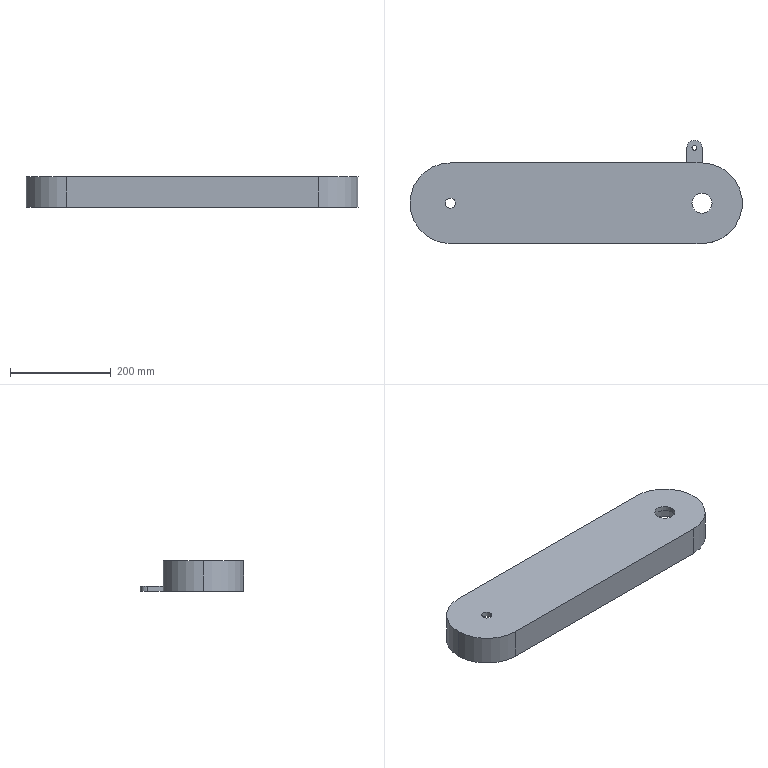Part | SolidWorks | features ICE 2, Extrusion 1 | 1 solid | 23 faces | box 660 x 205 x 60 mm | volume 1732722 mm3 | cylinder 13 | plane 10 | commonest cylinder face diameters 140 x3 160 x3 10 x2 20 x2 40 x2 30 x1
STEP:
#1=CARTESIAN_POINT('',(-10.,110.,-40.));
#2=VERTEX_POINT('',#1);
#3=CARTESIAN_POINT('',(-20.,110.,-40.));
#4=VERTEX_POINT('',#3);
#5=CARTESIAN_POINT('',(-15.,110.,-40.));
#6=DIRECTION('',(0.,0.,-1.));
#7=DIRECTION('',(-1.,0.,0.));
#8=AXIS2_PLACEMENT_3D('',#5,#6,#7);
#9=CIRCLE('',#8,5.);
#10=EDGE_CURVE('',#2,#4,#9,.T.);
#11=ORIENTED_EDGE('',*,*,#10,.F.);
#12=CARTESIAN_POINT('',(-10.,110.,-50.));
#13=VERTEX_POINT('',#12);
#14=CARTESIAN_POINT('',(-10.,110.,-40.));
#15=DIRECTION('',(0.,0.,-1.));
#16=VECTOR('',#15,1000.);
#17=LINE('',#14,#16);
#18=EDGE_CURVE('',#2,#13,#17,.T.);
#19=ORIENTED_EDGE('',*,*,#18,.T.);
#20=CARTESIAN_POINT('',(-20.,110.,-50.));
#21=VERTEX_POINT('',#20);
#22=CARTESIAN_POINT('',(-15.,110.,-50.));
#23=DIRECTION('',(0.,0.,-1.));
#24=DIRECTION('',(-1.,0.,0.));
#25=AXIS2_PLACEMENT_3D('',#22,#23,#24);
#26=CIRCLE('',#25,5.);
#27=EDGE_CURVE('',#13,#21,#26,.T.);
#28=ORIENTED_EDGE('',*,*,#27,.T.);
#29=CARTESIAN_POINT('',(-20.,110.,-40.));
#30=DIRECTION('',(0.,0.,-1.));
#31=VECTOR('',#30,1000.);
#32=LINE('',#29,#31);
#33=EDGE_CURVE('',#4,#21,#32,.T.);
#34=ORIENTED_EDGE('',*,*,#33,.F.);
#35=EDGE_LOOP('',(#11,#19,#28,#34));
#36=FACE_OUTER_BOUND('',#35,.T.);
#37=CARTESIAN_POINT('',(-15.,110.,-40.));
#38=DIRECTION('',(0.,0.,-1.));
#39=DIRECTION('',(-1.,0.,0.));
#40=AXIS2_PLACEMENT_3D('',#37,#38,#39);
#41=CYLINDRICAL_SURFACE('',#40,5.);
#42=ADVANCED_FACE('',(#36),#41,.F.);
#43=CARTESIAN_POINT('',(0.,70.,-50.));
#44=VERTEX_POINT('',#43);
#45=CARTESIAN_POINT('',(70.,0.,-50.));
#46=VERTEX_POINT('',#45);
#47=CARTESIAN_POINT('',(0.,0.,-50.));
#48=DIRECTION('',(0.,0.,-1.));
#49=DIRECTION('',(-1.,0.,0.));
#50=AXIS2_PLACEMENT_3D('',#47,#48,#49);
#51=CIRCLE('',#50,70.);
#52=EDGE_CURVE('',#44,#46,#51,.T.);
#53=ORIENTED_EDGE('',*,*,#52,.T.);
#54=CARTESIAN_POINT('',(70.,0.,0.));
#55=VERTEX_POINT('',#54);
#56=CARTESIAN_POINT('',(70.,0.,-50.));
#57=DIRECTION('',(0.,0.,1.));
#58=VECTOR('',#57,1000.);
#59=LINE('',#56,#58);
#60=EDGE_CURVE('',#46,#55,#59,.T.);
#61=ORIENTED_EDGE('',*,*,#60,.T.);
#62=CARTESIAN_POINT('',(0.,70.,0.));
#63=VERTEX_POINT('',#62);
#64=CARTESIAN_POINT('',(0.,0.,0.));
#65=DIRECTION('',(0.,0.,-1.));
#66=DIRECTION('',(-1.,0.,0.));
#67=AXIS2_PLACEMENT_3D('',#64,#65,#66);
#68=CIRCLE('',#67,70.);
#69=EDGE_CURVE('',#63,#55,#68,.T.);
#70=ORIENTED_EDGE('',*,*,#69,.F.);
#71=CARTESIAN_POINT('',(0.,70.,-50.));
#72=DIRECTION('',(0.,0.,1.));
#73=VECTOR('',#72,1000.);
#74=LINE('',#71,#73);
#75=EDGE_CURVE('',#44,#63,#74,.T.);
#76=ORIENTED_EDGE('',*,*,#75,.F.);
#77=EDGE_LOOP('',(#53,#61,#70,#76));
#78=FACE_OUTER_BOUND('',#77,.T.);
#79=CARTESIAN_POINT('',(0.,0.,-50.));
#80=DIRECTION('',(0.,0.,1.));
#81=DIRECTION('',(1.,0.,0.));
#82=AXIS2_PLACEMENT_3D('',#79,#80,#81);
#83=CYLINDRICAL_SURFACE('',#82,70.);
#84=ADVANCED_FACE('',(#78),#83,.F.);
#85=CARTESIAN_POINT('',(-510.,0.,10.));
#86=VERTEX_POINT('',#85);
#87=CARTESIAN_POINT('',(-490.,0.,10.));
#88=VERTEX_POINT('',#87);
#89=CARTESIAN_POINT('',(-500.,0.,10.));
#90=DIRECTION('',(0.,0.,1.));
#91=DIRECTION('',(1.,0.,0.));
#92=AXIS2_PLACEMENT_3D('',#89,#90,#91);
#93=CIRCLE('',#92,10.);
#94=EDGE_CURVE('',#86,#88,#93,.T.);
#95=ORIENTED_EDGE('',*,*,#94,.T.);
#96=CARTESIAN_POINT('',(-490.,0.,0.));
#97=VERTEX_POINT('',#96);
#98=CARTESIAN_POINT('',(-490.,0.,10.));
#99=DIRECTION('',(0.,0.,-1.));
#100=VECTOR('',#99,1000.);
#101=LINE('',#98,#100);
#102=EDGE_CURVE('',#88,#97,#101,.T.);
#103=ORIENTED_EDGE('',*,*,#102,.T.);
#104=CARTESIAN_POINT('',(-510.,0.,0.));
#105=VERTEX_POINT('',#104);
#106=CARTESIAN_POINT('',(-500.,0.,0.));
#107=DIRECTION('',(0.,0.,1.));
#108=DIRECTION('',(1.,0.,0.));
#109=AXIS2_PLACEMENT_3D('',#106,#107,#108);
#110=CIRCLE('',#109,10.);
#111=EDGE_CURVE('',#105,#97,#110,.T.);
#112=ORIENTED_EDGE('',*,*,#111,.F.);
#113=CARTESIAN_POINT('',(-510.,0.,10.));
#114=DIRECTION('',(0.,0.,-1.));
#115=VECTOR('',#114,1000.);
#116=LINE('',#113,#115);
#117=EDGE_CURVE('',#86,#105,#116,.T.);
#118=ORIENTED_EDGE('',*,*,#117,.F.);
#119=EDGE_LOOP('',(#95,#103,#112,#118));
#120=FACE_OUTER_BOUND('',#119,.T.);
#121=CARTESIAN_POINT('',(-500.,0.,10.));
#122=DIRECTION('',(0.,0.,-1.));
#123=DIRECTION('',(-1.,0.,0.));
#124=AXIS2_PLACEMENT_3D('',#121,#122,#123);
#125=CYLINDRICAL_SURFACE('',#124,10.);
#126=ADVANCED_FACE('',(#120),#125,.F.);
#127=CARTESIAN_POINT('',(-20.,0.,10.));
#128=VERTEX_POINT('',#127);
#129=CARTESIAN_POINT('',(20.,0.,10.));
#130=VERTEX_POINT('',#129);
#131=CARTESIAN_POINT('',(0.,0.,10.));
#132=DIRECTION('',(0.,0.,1.));
#133=DIRECTION('',(1.,0.,0.));
#134=AXIS2_PLACEMENT_3D('',#131,#132,#133);
#135=CIRCLE('',#134,20.);
#136=EDGE_CURVE('',#128,#130,#135,.T.);
#137=ORIENTED_EDGE('',*,*,#136,.T.);
#138=CARTESIAN_POINT('',(20.,0.,0.));
#139=VERTEX_POINT('',#138);
#140=CARTESIAN_POINT('',(20.,0.,10.));
#141=DIRECTION('',(0.,0.,-1.));
#142=VECTOR('',#141,1000.);
#143=LINE('',#140,#142);
#144=EDGE_CURVE('',#130,#139,#143,.T.);
#145=ORIENTED_EDGE('',*,*,#144,.T.);
#146=CARTESIAN_POINT('',(-20.,0.,0.));
#147=VERTEX_POINT('',#146);
#148=CARTESIAN_POINT('',(0.,0.,0.));
#149=DIRECTION('',(0.,0.,1.));
#150=DIRECTION('',(1.,0.,0.));
#151=AXIS2_PLACEMENT_3D('',#148,#149,#150);
#152=CIRCLE('',#151,20.);
#153=EDGE_CURVE('',#147,#139,#152,.T.);
#154=ORIENTED_EDGE('',*,*,#153,.F.);
#155=CARTESIAN_POINT('',(-20.,0.,10.));
#156=DIRECTION('',(0.,0.,-1.));
#157=VECTOR('',#156,1000.);
#158=LINE('',#155,#157);
#159=EDGE_CURVE('',#128,#147,#158,.T.);
#160=ORIENTED_EDGE('',*,*,#159,.F.);
#161=EDGE_LOOP('',(#137,#145,#154,#160));
#162=FACE_OUTER_BOUND('',#161,.T.);
#163=CARTESIAN_POINT('',(0.,0.,10.));
#164=DIRECTION('',(0.,0.,-1.));
#165=DIRECTION('',(-1.,0.,0.));
#166=AXIS2_PLACEMENT_3D('',#163,#164,#165);
#167=CYLINDRICAL_SURFACE('',#166,20.);
#168=ADVANCED_FACE('',(#162),#167,.F.);
#169=CARTESIAN_POINT('',(-580.,0.,10.));
#170=VERTEX_POINT('',#169);
#171=CARTESIAN_POINT('',(-500.,-80.,10.));
#172=VERTEX_POINT('',#171);
#173=CARTESIAN_POINT('',(-500.,0.,10.));
#174=DIRECTION('',(0.,0.,1.));
#175=DIRECTION('',(1.,0.,0.));
#176=AXIS2_PLACEMENT_3D('',#173,#174,#175);
#177=CIRCLE('',#176,80.);
#178=EDGE_CURVE('',#170,#172,#177,.T.);
#179=ORIENTED_EDGE('',*,*,#178,.F.);
#180=CARTESIAN_POINT('',(-580.,0.,-50.));
#181=VERTEX_POINT('',#180);
#182=CARTESIAN_POINT('',(-580.,0.,10.));
#183=DIRECTION('',(0.,0.,-1.));
#184=VECTOR('',#183,1000.);
#185=LINE('',#182,#184);
#186=EDGE_CURVE('',#170,#181,#185,.T.);
#187=ORIENTED_EDGE('',*,*,#186,.T.);
#188=CARTESIAN_POINT('',(-500.,-80.,-50.));
#189=VERTEX_POINT('',#188);
#190=CARTESIAN_POINT('',(-500.,0.,-50.));
#191=DIRECTION('',(0.,0.,-1.));
#192=DIRECTION('',(-1.,0.,0.));
#193=AXIS2_PLACEMENT_3D('',#190,#191,#192);
#194=CIRCLE('',#193,80.);
#195=EDGE_CURVE('',#189,#181,#194,.T.);
#196=ORIENTED_EDGE('',*,*,#195,.F.);
#197=CARTESIAN_POINT('',(-500.,-80.,10.));
#198=DIRECTION('',(0.,0.,-1.));
#199=VECTOR('',#198,1000.);
#200=LINE('',#197,#199);
#201=EDGE_CURVE('',#172,#189,#200,.T.);
#202=ORIENTED_EDGE('',*,*,#201,.F.);
#203=EDGE_LOOP('',(#179,#187,#196,#202));
#204=FACE_OUTER_BOUND('',#203,.T.);
#205=CARTESIAN_POINT('',(-500.,0.,10.));
#206=DIRECTION('',(0.,0.,-1.));
#207=DIRECTION('',(-1.,0.,0.));
#208=AXIS2_PLACEMENT_3D('',#205,#206,#207);
#209=CYLINDRICAL_SURFACE('',#208,80.);
#210=ADVANCED_FACE('',(#204),#209,.T.);
#211=ORIENTED_EDGE('',*,*,#136,.F.);
#212=CARTESIAN_POINT('',(0.,0.,10.));
#213=DIRECTION('',(0.,0.,1.));
#214=DIRECTION('',(1.,0.,0.));
#215=AXIS2_PLACEMENT_3D('',#212,#213,#214);
#216=CIRCLE('',#215,20.);
#217=EDGE_CURVE('',#130,#128,#216,.T.);
#218=ORIENTED_EDGE('',*,*,#217,.F.);
#219=EDGE_LOOP('',(#211,#218));
#220=FACE_BOUND('',#219,.T.);
#221=CARTESIAN_POINT('',(0.,-80.,10.));
#222=VERTEX_POINT('',#221);
#223=CARTESIAN_POINT('',(0.,80.,10.));
#224=VERTEX_POINT('',#223);
#225=CARTESIAN_POINT('',(0.,0.,10.));
#226=DIRECTION('',(0.,0.,1.));
#227=DIRECTION('',(1.,0.,0.));
#228=AXIS2_PLACEMENT_3D('',#225,#226,#227);
#229=CIRCLE('',#228,80.);
#230=EDGE_CURVE('',#222,#224,#229,.T.);
#231=ORIENTED_EDGE('',*,*,#230,.T.);
#232=CARTESIAN_POINT('',(-500.,80.,10.));
#233=VERTEX_POINT('',#232);
#234=CARTESIAN_POINT('',(0.,80.,10.));
#235=DIRECTION('',(-1.,0.,0.));
#236=VECTOR('',#235,1000.);
#237=LINE('',#234,#236);
#238=EDGE_CURVE('',#224,#233,#237,.T.);
#239=ORIENTED_EDGE('',*,*,#238,.T.);
#240=CARTESIAN_POINT('',(-500.,0.,10.));
#241=DIRECTION('',(0.,0.,1.));
#242=DIRECTION('',(1.,0.,0.));
#243=AXIS2_PLACEMENT_3D('',#240,#241,#242);
#244=CIRCLE('',#243,80.);
#245=EDGE_CURVE('',#233,#170,#244,.T.);
#246=ORIENTED_EDGE('',*,*,#245,.T.);
#247=ORIENTED_EDGE('',*,*,#178,.T.);
#248=CARTESIAN_POINT('',(-500.,-80.,10.));
#249=DIRECTION('',(1.,0.,0.));
#250=VECTOR('',#249,1000.);
#251=LINE('',#248,#250);
#252=EDGE_CURVE('',#172,#222,#251,.T.);
#253=ORIENTED_EDGE('',*,*,#252,.T.);
#254=EDGE_LOOP('',(#231,#239,#246,#247,#253));
#255=FACE_OUTER_BOUND('',#254,.T.);
#256=ORIENTED_EDGE('',*,*,#94,.F.);
#257=CARTESIAN_POINT('',(-500.,0.,10.));
#258=DIRECTION('',(0.,0.,1.));
#259=DIRECTION('',(1.,0.,0.));
#260=AXIS2_PLACEMENT_3D('',#257,#258,#259);
#261=CIRCLE('',#260,10.);
#262=EDGE_CURVE('',#88,#86,#261,.T.);
#263=ORIENTED_EDGE('',*,*,#262,.F.);
#264=EDGE_LOOP('',(#256,#263));
#265=FACE_BOUND('',#264,.T.);
#266=CARTESIAN_POINT('',(0.,0.,10.));
#267=DIRECTION('',(0.,0.,1.));
#268=DIRECTION('',(1.,0.,0.));
#269=AXIS2_PLACEMENT_3D('',#266,#267,#268);
#270=PLANE('',#269);
#271=ADVANCED_FACE('',(#220,#255,#265),#270,.T.);
#272=CARTESIAN_POINT('',(-500.,70.,0.));
#273=VERTEX_POINT('',#272);
#274=CARTESIAN_POINT('',(-500.,70.,0.));
#275=DIRECTION('',(1.,0.,0.));
#276=VECTOR('',#275,1000.);
#277=LINE('',#274,#276);
#278=EDGE_CURVE('',#273,#63,#277,.T.);
#279=ORIENTED_EDGE('',*,*,#278,.T.);
#280=ORIENTED_EDGE('',*,*,#69,.T.);
#281=CARTESIAN_POINT('',(0.,-70.,0.));
#282=VERTEX_POINT('',#281);
#283=CARTESIAN_POINT('',(0.,0.,0.));
#284=DIRECTION('',(0.,0.,-1.));
#285=DIRECTION('',(-1.,0.,0.));
#286=AXIS2_PLACEMENT_3D('',#283,#284,#285);
#287=CIRCLE('',#286,70.);
#288=EDGE_CURVE('',#55,#282,#287,.T.);
#289=ORIENTED_EDGE('',*,*,#288,.T.);
#290=CARTESIAN_POINT('',(-500.,-70.,0.));
#291=VERTEX_POINT('',#290);
#292=CARTESIAN_POINT('',(0.,-70.,0.));
#293=DIRECTION('',(-1.,0.,0.));
#294=VECTOR('',#293,1000.);
#295=LINE('',#292,#294);
#296=EDGE_CURVE('',#282,#291,#295,.T.);
#297=ORIENTED_EDGE('',*,*,#296,.T.);
#298=CARTESIAN_POINT('',(-500.,0.,0.));
#299=DIRECTION('',(0.,0.,-1.));
#300=DIRECTION('',(-1.,0.,0.));
#301=AXIS2_PLACEMENT_3D('',#298,#299,#300);
#302=CIRCLE('',#301,70.);
#303=EDGE_CURVE('',#291,#273,#302,.T.);
#304=ORIENTED_EDGE('',*,*,#303,.T.);
#305=EDGE_LOOP('',(#279,#280,#289,#297,#304));
#306=FACE_OUTER_BOUND('',#305,.T.);
#307=ORIENTED_EDGE('',*,*,#153,.T.);
#308=CARTESIAN_POINT('',(0.,0.,0.));
#309=DIRECTION('',(0.,0.,1.));
#310=DIRECTION('',(1.,0.,0.));
#311=AXIS2_PLACEMENT_3D('',#308,#309,#310);
#312=CIRCLE('',#311,20.);
#313=EDGE_CURVE('',#139,#147,#312,.T.);
#314=ORIENTED_EDGE('',*,*,#313,.T.);
#315=EDGE_LOOP('',(#307,#314));
#316=FACE_BOUND('',#315,.T.);
#317=ORIENTED_EDGE('',*,*,#111,.T.);
#318=CARTESIAN_POINT('',(-500.,0.,0.));
#319=DIRECTION('',(0.,0.,1.));
#320=DIRECTION('',(1.,0.,0.));
#321=AXIS2_PLACEMENT_3D('',#318,#319,#320);
#322=CIRCLE('',#321,10.);
#323=EDGE_CURVE('',#97,#105,#322,.T.);
#324=ORIENTED_EDGE('',*,*,#323,.T.);
#325=EDGE_LOOP('',(#317,#324));
#326=FACE_BOUND('',#325,.T.);
#327=CARTESIAN_POINT('',(0.,0.,0.));
#328=DIRECTION('',(0.,0.,1.));
#329=DIRECTION('',(1.,0.,0.));
#330=AXIS2_PLACEMENT_3D('',#327,#328,#329);
#331=PLANE('',#330);
#332=ADVANCED_FACE('',(#306,#316,#326),#331,.F.);
#333=CARTESIAN_POINT('',(0.,-80.,-50.));
#334=VERTEX_POINT('',#333);
#335=CARTESIAN_POINT('',(0.,-80.,10.));
#336=DIRECTION('',(0.,0.,-1.));
#337=VECTOR('',#336,1000.);
#338=LINE('',#335,#337);
#339=EDGE_CURVE('',#222,#334,#338,.T.);
#340=ORIENTED_EDGE('',*,*,#339,.T.);
#341=CARTESIAN_POINT('',(0.,80.,-50.));
#342=VERTEX_POINT('',#341);
#343=CARTESIAN_POINT('',(0.,0.,-50.));
#344=DIRECTION('',(0.,0.,-1.));
#345=DIRECTION('',(-1.,0.,0.));
#346=AXIS2_PLACEMENT_3D('',#343,#344,#345);
#347=CIRCLE('',#346,80.);
#348=EDGE_CURVE('',#342,#334,#347,.T.);
#349=ORIENTED_EDGE('',*,*,#348,.F.);
#350=CARTESIAN_POINT('',(0.,80.,-40.));
#351=VERTEX_POINT('',#350);
#352=CARTESIAN_POINT('',(0.,80.,-40.));
#353=DIRECTION('',(0.,0.,-1.));
#354=VECTOR('',#353,1000.);
#355=LINE('',#352,#354);
#356=EDGE_CURVE('',#351,#342,#355,.T.);
#357=ORIENTED_EDGE('',*,*,#356,.F.);
#358=CARTESIAN_POINT('',(0.,80.,10.));
#359=DIRECTION('',(0.,0.,-1.));
#360=VECTOR('',#359,1000.);
#361=LINE('',#358,#360);
#362=EDGE_CURVE('',#224,#351,#361,.T.);
#363=ORIENTED_EDGE('',*,*,#362,.F.);
#364=ORIENTED_EDGE('',*,*,#230,.F.);
#365=EDGE_LOOP('',(#340,#349,#357,#363,#364));
#366=FACE_OUTER_BOUND('',#365,.T.);
#367=CARTESIAN_POINT('',(0.,0.,10.));
#368=DIRECTION('',(0.,0.,-1.));
#369=DIRECTION('',(-1.,0.,0.));
#370=AXIS2_PLACEMENT_3D('',#367,#368,#369);
#371=CYLINDRICAL_SURFACE('',#370,80.);
#372=ADVANCED_FACE('',(#366),#371,.T.);
#373=CARTESIAN_POINT('',(-30.,80.,-40.));
#374=VERTEX_POINT('',#373);
#375=CARTESIAN_POINT('',(0.,80.,-40.));
#376=DIRECTION('',(-1.,0.,0.));
#377=VECTOR('',#376,1000.);
#378=LINE('',#375,#377);
#379=EDGE_CURVE('',#351,#374,#378,.T.);
#380=ORIENTED_EDGE('',*,*,#379,.T.);
#381=CARTESIAN_POINT('',(-30.,80.,-50.));
#382=VERTEX_POINT('',#381);
#383=CARTESIAN_POINT('',(-30.,80.,-40.));
#384=DIRECTION('',(0.,0.,-1.));
#385=VECTOR('',#384,1000.);
#386=LINE('',#383,#385);
#387=EDGE_CURVE('',#374,#382,#386,.T.);
#388=ORIENTED_EDGE('',*,*,#387,.T.);
#389=CARTESIAN_POINT('',(-500.,80.,-50.));
#390=VERTEX_POINT('',#389);
#391=CARTESIAN_POINT('',(-500.,80.,-50.));
#392=DIRECTION('',(1.,0.,0.));
#393=VECTOR('',#392,1000.);
#394=LINE('',#391,#393);
#395=EDGE_CURVE('',#390,#382,#394,.T.);
#396=ORIENTED_EDGE('',*,*,#395,.F.);
#397=CARTESIAN_POINT('',(-500.,80.,10.));
#398=DIRECTION('',(0.,0.,-1.));
#399=VECTOR('',#398,1000.);
#400=LINE('',#397,#399);
#401=EDGE_CURVE('',#233,#390,#400,.T.);
#402=ORIENTED_EDGE('',*,*,#401,.F.);
#403=ORIENTED_EDGE('',*,*,#238,.F.);
#404=ORIENTED_EDGE('',*,*,#362,.T.);
#405=EDGE_LOOP('',(#380,#388,#396,#402,#403,#404));
#406=FACE_OUTER_BOUND('',#405,.T.);
#407=CARTESIAN_POINT('',(0.,80.,10.));
#408=DIRECTION('',(0.,-1.,0.));
#409=DIRECTION('',(1.,0.,0.));
#410=AXIS2_PLACEMENT_3D('',#407,#408,#409);
#411=PLANE('',#410);
#412=ADVANCED_FACE('',(#406),#411,.F.);
#413=ORIENTED_EDGE('',*,*,#186,.F.);
#414=ORIENTED_EDGE('',*,*,#245,.F.);
#415=ORIENTED_EDGE('',*,*,#401,.T.);
#416=CARTESIAN_POINT('',(-500.,0.,-50.));
#417=DIRECTION('',(0.,0.,-1.));
#418=DIRECTION('',(-1.,0.,0.));
#419=AXIS2_PLACEMENT_3D('',#416,#417,#418);
#420=CIRCLE('',#419,80.);
#421=EDGE_CURVE('',#181,#390,#420,.T.);
#422=ORIENTED_EDGE('',*,*,#421,.F.);
#423=EDGE_LOOP('',(#413,#414,#415,#422));
#424=FACE_OUTER_BOUND('',#423,.T.);
#425=CARTESIAN_POINT('',(-500.,0.,10.));
#426=DIRECTION('',(0.,0.,-1.));
#427=DIRECTION('',(-1.,0.,0.));
#428=AXIS2_PLACEMENT_3D('',#425,#426,#427);
#429=CYLINDRICAL_SURFACE('',#428,80.);
#430=ADVANCED_FACE('',(#424),#429,.T.);
#431=ORIENTED_EDGE('',*,*,#201,.T.);
#432=CARTESIAN_POINT('',(0.,-80.,-50.));
#433=DIRECTION('',(-1.,0.,0.));
#434=VECTOR('',#433,1000.);
#435=LINE('',#432,#434);
#436=EDGE_CURVE('',#334,#189,#435,.T.);
#437=ORIENTED_EDGE('',*,*,#436,.F.);
#438=ORIENTED_EDGE('',*,*,#339,.F.);
#439=ORIENTED_EDGE('',*,*,#252,.F.);
#440=EDGE_LOOP('',(#431,#437,#438,#439));
#441=FACE_OUTER_BOUND('',#440,.T.);
#442=CARTESIAN_POINT('',(-500.,-80.,10.));
#443=DIRECTION('',(0.,1.,0.));
#444=DIRECTION('',(0.,0.,1.));
#445=AXIS2_PLACEMENT_3D('',#442,#443,#444);
#446=PLANE('',#445);
#447=ADVANCED_FACE('',(#441),#446,.F.);
#448=ORIENTED_EDGE('',*,*,#144,.F.);
#449=ORIENTED_EDGE('',*,*,#217,.T.);
#450=ORIENTED_EDGE('',*,*,#159,.T.);
#451=ORIENTED_EDGE('',*,*,#313,.F.);
#452=EDGE_LOOP('',(#448,#449,#450,#451));
#453=FACE_OUTER_BOUND('',#452,.T.);
#454=CARTESIAN_POINT('',(0.,0.,10.));
#455=DIRECTION('',(0.,0.,-1.));
#456=DIRECTION('',(-1.,0.,0.));
#457=AXIS2_PLACEMENT_3D('',#454,#455,#456);
#458=CYLINDRICAL_SURFACE('',#457,20.);
#459=ADVANCED_FACE('',(#453),#458,.F.);
#460=ORIENTED_EDGE('',*,*,#102,.F.);
#461=ORIENTED_EDGE('',*,*,#262,.T.);
#462=ORIENTED_EDGE('',*,*,#117,.T.);
#463=ORIENTED_EDGE('',*,*,#323,.F.);
#464=EDGE_LOOP('',(#460,#461,#462,#463));
#465=FACE_OUTER_BOUND('',#464,.T.);
#466=CARTESIAN_POINT('',(-500.,0.,10.));
#467=DIRECTION('',(0.,0.,-1.));
#468=DIRECTION('',(-1.,0.,0.));
#469=AXIS2_PLACEMENT_3D('',#466,#467,#468);
#470=CYLINDRICAL_SURFACE('',#469,10.);
#471=ADVANCED_FACE('',(#465),#470,.F.);
#472=ORIENTED_EDGE('',*,*,#348,.T.);
#473=ORIENTED_EDGE('',*,*,#436,.T.);
#474=ORIENTED_EDGE('',*,*,#195,.T.);
#475=ORIENTED_EDGE('',*,*,#421,.T.);
#476=ORIENTED_EDGE('',*,*,#395,.T.);
#477=CARTESIAN_POINT('',(-30.,110.,-50.));
#478=VERTEX_POINT('',#477);
#479=CARTESIAN_POINT('',(-30.,110.,-50.));
#480=DIRECTION('',(0.,1.,0.));
#481=VECTOR('',#480,1000.);
#482=LINE('',#479,#481);
#483=EDGE_CURVE('',#382,#478,#482,.T.);
#484=ORIENTED_EDGE('',*,*,#483,.T.);
#485=CARTESIAN_POINT('',(0.,110.,-50.));
#486=VERTEX_POINT('',#485);
#487=CARTESIAN_POINT('',(-15.,110.,-50.));
#488=DIRECTION('',(0.,0.,-1.));
#489=DIRECTION('',(-1.,0.,0.));
#490=AXIS2_PLACEMENT_3D('',#487,#488,#489);
#491=CIRCLE('',#490,15.);
#492=EDGE_CURVE('',#478,#486,#491,.T.);
#493=ORIENTED_EDGE('',*,*,#492,.T.);
#494=CARTESIAN_POINT('',(0.,110.,-50.));
#495=DIRECTION('',(0.,-1.,0.));
#496=VECTOR('',#495,1000.);
#497=LINE('',#494,#496);
#498=EDGE_CURVE('',#486,#342,#497,.T.);
#499=ORIENTED_EDGE('',*,*,#498,.T.);
#500=EDGE_LOOP('',(#472,#473,#474,#475,#476,#484,#493,#499));
#501=FACE_OUTER_BOUND('',#500,.T.);
#502=CARTESIAN_POINT('',(0.,-70.,-50.));
#503=VERTEX_POINT('',#502);
#504=CARTESIAN_POINT('',(-500.,-70.,-50.));
#505=VERTEX_POINT('',#504);
#506=CARTESIAN_POINT('',(0.,-70.,-50.));
#507=DIRECTION('',(-1.,0.,0.));
#508=VECTOR('',#507,1000.);
#509=LINE('',#506,#508);
#510=EDGE_CURVE('',#503,#505,#509,.T.);
#511=ORIENTED_EDGE('',*,*,#510,.F.);
#512=CARTESIAN_POINT('',(0.,0.,-50.));
#513=DIRECTION('',(0.,0.,-1.));
#514=DIRECTION('',(-1.,0.,0.));
#515=AXIS2_PLACEMENT_3D('',#512,#513,#514);
#516=CIRCLE('',#515,70.);
#517=EDGE_CURVE('',#46,#503,#516,.T.);
#518=ORIENTED_EDGE('',*,*,#517,.F.);
#519=ORIENTED_EDGE('',*,*,#52,.F.);
#520=CARTESIAN_POINT('',(-500.,70.,-50.));
#521=VERTEX_POINT('',#520);
#522=CARTESIAN_POINT('',(-500.,70.,-50.));
#523=DIRECTION('',(1.,0.,0.));
#524=VECTOR('',#523,1000.);
#525=LINE('',#522,#524);
#526=EDGE_CURVE('',#521,#44,#525,.T.);
#527=ORIENTED_EDGE('',*,*,#526,.F.);
#528=CARTESIAN_POINT('',(-500.,0.,-50.));
#529=DIRECTION('',(0.,0.,-1.));
#530=DIRECTION('',(-1.,0.,0.));
#531=AXIS2_PLACEMENT_3D('',#528,#529,#530);
#532=CIRCLE('',#531,70.);
#533=EDGE_CURVE('',#505,#521,#532,.T.);
#534=ORIENTED_EDGE('',*,*,#533,.F.);
#535=EDGE_LOOP('',(#511,#518,#519,#527,#534));
#536=FACE_BOUND('',#535,.T.);
#537=CARTESIAN_POINT('',(-15.,110.,-50.));
#538=DIRECTION('',(0.,0.,-1.));
#539=DIRECTION('',(-1.,0.,0.));
#540=AXIS2_PLACEMENT_3D('',#537,#538,#539);
#541=CIRCLE('',#540,5.);
#542=EDGE_CURVE('',#21,#13,#541,.T.);
#543=ORIENTED_EDGE('',*,*,#542,.F.);
#544=ORIENTED_EDGE('',*,*,#27,.F.);
#545=EDGE_LOOP('',(#543,#544));
#546=FACE_BOUND('',#545,.T.);
#547=CARTESIAN_POINT('',(0.,0.,-50.));
#548=DIRECTION('',(0.,0.,-1.));
#549=DIRECTION('',(-1.,0.,0.));
#550=AXIS2_PLACEMENT_3D('',#547,#548,#549);
#551=PLANE('',#550);
#552=ADVANCED_FACE('',(#501,#536,#546),#551,.T.);
#553=ORIENTED_EDGE('',*,*,#60,.F.);
#554=ORIENTED_EDGE('',*,*,#517,.T.);
#555=CARTESIAN_POINT('',(0.,-70.,-50.));
#556=DIRECTION('',(0.,0.,1.));
#557=VECTOR('',#556,1000.);
#558=LINE('',#555,#557);
#559=EDGE_CURVE('',#503,#282,#558,.T.);
#560=ORIENTED_EDGE('',*,*,#559,.T.);
#561=ORIENTED_EDGE('',*,*,#288,.F.);
#562=EDGE_LOOP('',(#553,#554,#560,#561));
#563=FACE_OUTER_BOUND('',#562,.T.);
#564=CARTESIAN_POINT('',(0.,0.,-50.));
#565=DIRECTION('',(0.,0.,1.));
#566=DIRECTION('',(1.,0.,0.));
#567=AXIS2_PLACEMENT_3D('',#564,#565,#566);
#568=CYLINDRICAL_SURFACE('',#567,70.);
#569=ADVANCED_FACE('',(#563),#568,.F.);
#570=ORIENTED_EDGE('',*,*,#296,.F.);
#571=ORIENTED_EDGE('',*,*,#559,.F.);
#572=ORIENTED_EDGE('',*,*,#510,.T.);
#573=CARTESIAN_POINT('',(-500.,-70.,-50.));
#574=DIRECTION('',(0.,0.,1.));
#575=VECTOR('',#574,1000.);
#576=LINE('',#573,#575);
#577=EDGE_CURVE('',#505,#291,#576,.T.);
#578=ORIENTED_EDGE('',*,*,#577,.T.);
#579=EDGE_LOOP('',(#570,#571,#572,#578));
#580=FACE_OUTER_BOUND('',#579,.T.);
#581=CARTESIAN_POINT('',(0.,-70.,-50.));
#582=DIRECTION('',(0.,1.,0.));
#583=DIRECTION('',(-1.,0.,0.));
#584=AXIS2_PLACEMENT_3D('',#581,#582,#583);
#585=PLANE('',#584);
#586=ADVANCED_FACE('',(#580),#585,.T.);
#587=ORIENTED_EDGE('',*,*,#303,.F.);
#588=ORIENTED_EDGE('',*,*,#577,.F.);
#589=ORIENTED_EDGE('',*,*,#533,.T.);
#590=CARTESIAN_POINT('',(-500.,70.,-50.));
#591=DIRECTION('',(0.,0.,1.));
#592=VECTOR('',#591,1000.);
#593=LINE('',#590,#592);
#594=EDGE_CURVE('',#521,#273,#593,.T.);
#595=ORIENTED_EDGE('',*,*,#594,.T.);
#596=EDGE_LOOP('',(#587,#588,#589,#595));
#597=FACE_OUTER_BOUND('',#596,.T.);
#598=CARTESIAN_POINT('',(-500.,0.,-50.));
#599=DIRECTION('',(0.,0.,1.));
#600=DIRECTION('',(1.,0.,0.));
#601=AXIS2_PLACEMENT_3D('',#598,#599,#600);
#602=CYLINDRICAL_SURFACE('',#601,70.);
#603=ADVANCED_FACE('',(#597),#602,.F.);
#604=ORIENTED_EDGE('',*,*,#278,.F.);
#605=ORIENTED_EDGE('',*,*,#594,.F.);
#606=ORIENTED_EDGE('',*,*,#526,.T.);
#607=ORIENTED_EDGE('',*,*,#75,.T.);
#608=EDGE_LOOP('',(#604,#605,#606,#607));
#609=FACE_OUTER_BOUND('',#608,.T.);
#610=CARTESIAN_POINT('',(-500.,70.,-50.));
#611=DIRECTION('',(0.,-1.,0.));
#612=DIRECTION('',(1.,0.,0.));
#613=AXIS2_PLACEMENT_3D('',#610,#611,#612);
#614=PLANE('',#613);
#615=ADVANCED_FACE('',(#609),#614,.T.);
#616=ORIENTED_EDGE('',*,*,#483,.F.);
#617=ORIENTED_EDGE('',*,*,#387,.F.);
#618=CARTESIAN_POINT('',(-30.,110.,-40.));
#619=VERTEX_POINT('',#618);
#620=CARTESIAN_POINT('',(-30.,110.,-40.));
#621=DIRECTION('',(0.,1.,0.));
#622=VECTOR('',#621,1000.);
#623=LINE('',#620,#622);
#624=EDGE_CURVE('',#374,#619,#623,.T.);
#625=ORIENTED_EDGE('',*,*,#624,.T.);
#626=CARTESIAN_POINT('',(-30.,110.,-40.));
#627=DIRECTION('',(0.,0.,-1.));
#628=VECTOR('',#627,1000.);
#629=LINE('',#626,#628);
#630=EDGE_CURVE('',#619,#478,#629,.T.);
#631=ORIENTED_EDGE('',*,*,#630,.T.);
#632=EDGE_LOOP('',(#616,#617,#625,#631));
#633=FACE_OUTER_BOUND('',#632,.T.);
#634=CARTESIAN_POINT('',(-30.,110.,-40.));
#635=DIRECTION('',(-1.,0.,0.));
#636=DIRECTION('',(0.,-1.,0.));
#637=AXIS2_PLACEMENT_3D('',#634,#635,#636);
#638=PLANE('',#637);
#639=ADVANCED_FACE('',(#633),#638,.T.);
#640=ORIENTED_EDGE('',*,*,#498,.F.);
#641=CARTESIAN_POINT('',(0.,110.,-40.));
#642=VERTEX_POINT('',#641);
#643=CARTESIAN_POINT('',(0.,110.,-40.));
#644=DIRECTION('',(0.,0.,-1.));
#645=VECTOR('',#644,1000.);
#646=LINE('',#643,#645);
#647=EDGE_CURVE('',#642,#486,#646,.T.);
#648=ORIENTED_EDGE('',*,*,#647,.F.);
#649=CARTESIAN_POINT('',(0.,110.,-40.));
#650=DIRECTION('',(0.,-1.,0.));
#651=VECTOR('',#650,1000.);
#652=LINE('',#649,#651);
#653=EDGE_CURVE('',#642,#351,#652,.T.);
#654=ORIENTED_EDGE('',*,*,#653,.T.);
#655=ORIENTED_EDGE('',*,*,#356,.T.);
#656=EDGE_LOOP('',(#640,#648,#654,#655));
#657=FACE_OUTER_BOUND('',#656,.T.);
#658=CARTESIAN_POINT('',(0.,110.,-40.));
#659=DIRECTION('',(1.,0.,0.));
#660=DIRECTION('',(0.,0.,-1.));
#661=AXIS2_PLACEMENT_3D('',#658,#659,#660);
#662=PLANE('',#661);
#663=ADVANCED_FACE('',(#657),#662,.T.);
#664=ORIENTED_EDGE('',*,*,#492,.F.);
#665=ORIENTED_EDGE('',*,*,#630,.F.);
#666=CARTESIAN_POINT('',(-15.,110.,-40.));
#667=DIRECTION('',(0.,0.,-1.));
#668=DIRECTION('',(-1.,0.,0.));
#669=AXIS2_PLACEMENT_3D('',#666,#667,#668);
#670=CIRCLE('',#669,15.);
#671=EDGE_CURVE('',#619,#642,#670,.T.);
#672=ORIENTED_EDGE('',*,*,#671,.T.);
#673=ORIENTED_EDGE('',*,*,#647,.T.);
#674=EDGE_LOOP('',(#664,#665,#672,#673));
#675=FACE_OUTER_BOUND('',#674,.T.);
#676=CARTESIAN_POINT('',(-15.,110.,-40.));
#677=DIRECTION('',(0.,0.,-1.));
#678=DIRECTION('',(-1.,0.,0.));
#679=AXIS2_PLACEMENT_3D('',#676,#677,#678);
#680=CYLINDRICAL_SURFACE('',#679,15.);
#681=ADVANCED_FACE('',(#675),#680,.T.);
#682=CARTESIAN_POINT('',(-15.,110.,-40.));
#683=DIRECTION('',(0.,0.,-1.));
#684=DIRECTION('',(-1.,0.,0.));
#685=AXIS2_PLACEMENT_3D('',#682,#683,#684);
#686=CIRCLE('',#685,5.);
#687=EDGE_CURVE('',#4,#2,#686,.T.);
#688=ORIENTED_EDGE('',*,*,#687,.T.);
#689=ORIENTED_EDGE('',*,*,#10,.T.);
#690=EDGE_LOOP('',(#688,#689));
#691=FACE_BOUND('',#690,.T.);
#692=ORIENTED_EDGE('',*,*,#624,.F.);
#693=ORIENTED_EDGE('',*,*,#379,.F.);
#694=ORIENTED_EDGE('',*,*,#653,.F.);
#695=ORIENTED_EDGE('',*,*,#671,.F.);
#696=EDGE_LOOP('',(#692,#693,#694,#695));
#697=FACE_OUTER_BOUND('',#696,.T.);
#698=CARTESIAN_POINT('',(-15.,110.,-40.));
#699=DIRECTION('',(0.,0.,-1.));
#700=DIRECTION('',(-1.,0.,0.));
#701=AXIS2_PLACEMENT_3D('',#698,#699,#700);
#702=PLANE('',#701);
#703=ADVANCED_FACE('',(#691,#697),#702,.F.);
#704=ORIENTED_EDGE('',*,*,#18,.F.);
#705=ORIENTED_EDGE('',*,*,#687,.F.);
#706=ORIENTED_EDGE('',*,*,#33,.T.);
#707=ORIENTED_EDGE('',*,*,#542,.T.);
#708=EDGE_LOOP('',(#704,#705,#706,#707));
#709=FACE_OUTER_BOUND('',#708,.T.);
#710=CARTESIAN_POINT('',(-15.,110.,-40.));
#711=DIRECTION('',(0.,0.,-1.));
#712=DIRECTION('',(-1.,0.,0.));
#713=AXIS2_PLACEMENT_3D('',#710,#711,#712);
#714=CYLINDRICAL_SURFACE('',#713,5.);
#715=ADVANCED_FACE('',(#709),#714,.F.);
#716=CLOSED_SHELL('',(#42,#84,#126,#168,#210,#271,#332,#372,#412,#430,#447,#459,#471,#552,#569,#586,#603,#615,#639,#663,#681,#703,#715));
#717=MANIFOLD_SOLID_BREP('',#716);
#718=CARTESIAN_POINT('',(0.,0.,0.));
#719=DIRECTION('',(0.,0.,1.));
#720=DIRECTION('',(1.,0.,0.));
#721=AXIS2_PLACEMENT_3D('',#718,#719,#720);
#722=(LENGTH_UNIT()NAMED_UNIT(*)SI_UNIT(.MILLI.,.METRE.));
#723=UNCERTAINTY_MEASURE_WITH_UNIT(LENGTH_MEASURE(0.00001),#722,'','');
#724=(NAMED_UNIT(*)PLANE_ANGLE_UNIT()SI_UNIT($,.RADIAN.));
#725=(NAMED_UNIT(*)SI_UNIT($,.STERADIAN.)SOLID_ANGLE_UNIT());
#726=(GEOMETRIC_REPRESENTATION_CONTEXT(3)GLOBAL_UNCERTAINTY_ASSIGNED_CONTEXT((#723))GLOBAL_UNIT_ASSIGNED_CONTEXT((#722,#724,#725))REPRESENTATION_CONTEXT('',''));
#727=ADVANCED_BREP_SHAPE_REPRESENTATION('',(#717,#721),#726);